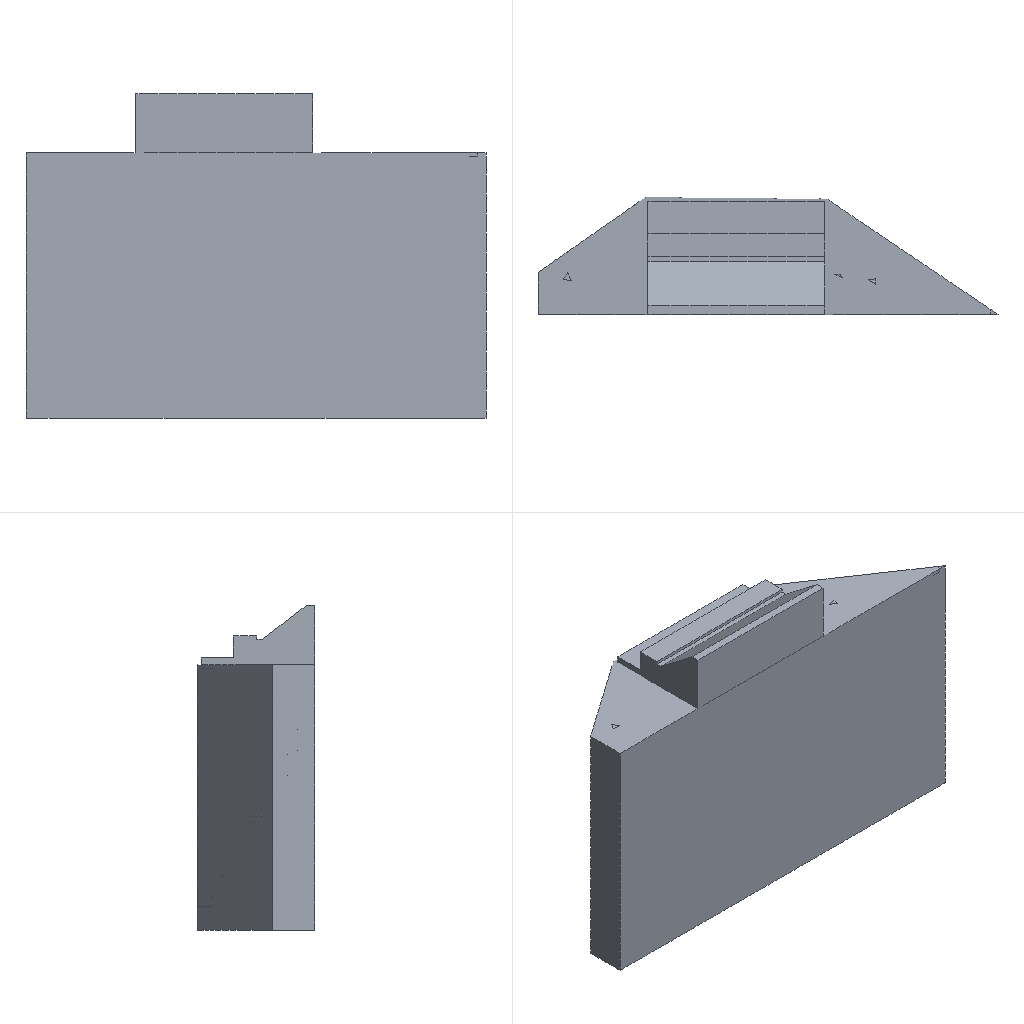Simulation study | ansys workbench
Set-up summary:
category,name,step,type,value,unit,region
solver,ansys_workbench
units,mm-N-s-tonne (MPa),,stated,"/units,MPA"
analysis,LS1,,static
load_step,LS1,LS1,static,nsubst=1; time=1
mesh,nodes,,,241341
mesh,elements,,,176783
element_type,SOLID187,,,141912
element_type,TARGE170,,,14127
element_type,CONTA174,,,14127
element_type,SOLID186,,,5881
element_type,SURF154,,,736
material,AC-16,,E,1300,tonne s^-2 mm^-1
material,AC-16,,nu,0.3
material,AC-16,,density,2.44e-09,tonne mm^-3
material,Water ?,,E,60,tonne s^-2 mm^-1
material,Water ?,,nu,0.3
material,Water ?,,density,1.9e-09,tonne mm^-3
material,C30,,E,30000,tonne s^-2 mm^-1
material,C30,,nu,0.2
material,C30,,density,2.6e-09,tonne mm^-3
material,SAM-13,,E,1800,tonne s^-2 mm^-1
material,SAM-13,,nu,0.33
material,SAM-13,,density,2.46e-09,tonne mm^-3
load,"Define Pressure Using Surface Effect Elements ""__""",LS1,pressure,0.5,,SURF154 #45
load,ACEL,LS1,gravity (ACEL; gravity acts opposite),"9806.65 [dir=(0, -1, 0)]",,all
bc,Fixed Supports,model,fixed,[dofs=ALL],,_FIXEDSU
contact,Contact Region,,bonded (always),element=CONTA174
contact,Contact Region 2,,bonded (always),element=CONTA174
contact,Contact Region 3,,bonded (always),element=CONTA174
contact,Contact Region 4,,bonded (always),element=CONTA174
contact,Contact Region 5,,bonded (always),element=CONTA174
contact,Contact Region 6,,bonded (always),element=CONTA174
contact,Contact Region 7,,bonded (always),element=CONTA174
contact,Contact Region 8,,bonded (always),element=CONTA174
contact,Contact Region 9,,bonded (always),element=CONTA174
contact,Contact Region 10,,bonded (always),element=CONTA174
contact,Contact Region 11,,bonded (always),element=CONTA174
contact,Contact Region 12,,bonded (always),element=CONTA174
contact,Contact Region 13,,bonded (always),element=CONTA174
contact,Contact Region 14,,bonded (always),element=CONTA174
contact,Contact Region 15,,bonded (always),element=CONTA174
contact,Contact Region 16,,bonded (always),element=CONTA174
contact,Contact Region 17,,bonded (always),element=CONTA174
named_set,_FIXEDSU,,node,7961
Ansys APDL input file, long lists of numbers shortened:
/batch
/config,noeldb,1     ! force off writing results to database
*get,_wallstrt,active,,time,wall
! ANSYS input file written by Workbench version 2024 R2
! File used for geometry attach:
/title,__--____ (A5)
! ****** Begin Custom Load Command Snippet ******
/COM, ACT Extensions:
/COM,     LSDYNA, 2024.2
/COM,/COM,     ANSYSMotion, 2024.2
/COM,
! ****** End   Custom Load Command Snippet ******
/com,--- Data in consistent NMM units. See Solving Units in the help system for more information.
/units,MPA
/nopr
/wb,file,start              !  signify a WB generated input file
/prep7
! Turn off shape checking because checks already performed inside WB mesher.
! See help system for more information.
SHPP,OFF,,NOWARN
/nolist
etcon,set             ! allow ANSYS to choose best KEYOP's for 180x elements, resets any applicable keyopt to MAPDL defaults
/com,*********** Nodes for the whole assembly ***********
nblock,3,,265475
(1i9,3e20.9e3)
   141650     3.031677267E+02     6.841687785E+02    -6.937544574E+02
! (241340 more lines like these left out)
-1
/wb,elem,start            !  set before creation of elements
/com,*********** Elements for Body 1 '62110001-FreeParts|__4[7]' ***********
et,1,186
keyo,1,2,1          ! set full integration on SOLID186
eblock,19,solid,,144
(19i9)
        1        1        1        1        0        0        0        0       20        0        1        1      194      199      201       92      195      200      224
! (287 more lines like these left out)
-1
/com,*********** Elements for Body 2 '62110001-FreeParts|__4[6]' ***********
et,2,186
keyo,2,2,1          ! set full integration on SOLID186
eblock,19,solid,,208
(19i9)
        2        2        2        2        0        0        0        0       20        0      145     1285     1317     1366     1392     1289     1316     1367     1393
! (415 more lines like these left out)
-1
/com,*********** Elements for Body 3 '62110001-FreeParts|__2' ***********
et,3,186
keyo,3,2,1          ! set full integration on SOLID186
eblock,19,solid,,1302
(19i9)
        3        3        3        3        0        0        0        0       20        0      353     3709     4247     4329     3762     3742     4307     4330     3763
! (2603 more lines like these left out)
-1
/com,*********** Elements for Body 4 '62110001-FreeParts|__4[2]' ***********
et,4,186
keyo,4,2,1          ! set full integration on SOLID186
eblock,19,solid,,1508
(19i9)
        4        4        4        4        0        0        0        0       20        0     1655     9285    11532    11587    11716     9986    11585    11586    11741
! (3015 more lines like these left out)
-1
/com,*********** Elements for Body 5 '62110001-FreeParts|__4[3]' ***********
et,5,186
keyo,5,2,1          ! set full integration on SOLID186
eblock,19,solid,,1392
(19i9)
        5        5        5        5        0        0        0        0       20        0     3163    18104    20284    20200    20142    19391    20307    20201    20170
! (2783 more lines like these left out)
-1
/com,*********** Elements for Body 6 '62110001-FreeParts|__3[6]' ***********
et,6,186
keyo,6,2,1          ! set full integration on SOLID186
eblock,19,solid,,591
(19i9)
        6        6        6        6        0        0        0        0       20        0     4555    26309    26310    26422    26421    27122    27121    27009    27010
! (1181 more lines like these left out)
-1
/com,*********** Elements for Body 7 '62110001-FreeParts|__4[5]' ***********
et,7,187
eblock,19,solid,,73405
(19i9)
        7        7        7        7        0        0        0        0       10        0     5146    37364    44991    40740    42244    97102   123084    97095    97098
! (146809 more lines like these left out)
-1
/com,*********** Elements for Body 8 '62110001-FreeParts|__4[4]' ***********
et,8,186
keyo,8,2,1          ! set full integration on SOLID186
eblock,19,solid,,667
(19i9)
        8        8        8        8        0        0        0        0       20        0    78551   137333   138129   138101   138099   137334   138005   138006   138007
! (1333 more lines like these left out)
-1
/com,*********** Elements for Body 9 '62110001-FreeParts|__4[8]' ***********
et,9,186
keyo,9,2,1          ! set full integration on SOLID186
eblock,19,solid,,69
(19i9)
        9        9        9        9        0        0        0        0       20        0    79218   141693   141815   141816   141817   141694   141764   141765   141740
! (137 more lines like these left out)
-1
/com,*********** Elements for Body 10 '62110001-FreeParts|__4[1]' ***********
et,10,187
eblock,19,solid,,68507
(19i9)
       10       10       10       10        0        0        0        0       10        0    79287   149696   150014   155698   150959   212844   215335   212849   212847
! (137013 more lines like these left out)
-1
/wb,elem,end               !  done creating elements
/com,*********** Send User Defined Coordinate System(s) ***********
csys,0
toffst,273.15,      ! Temperature offset from absolute zero
/com,*********** Set Reference Temperature ***********
tref,22.
/wb,mat,start              !  starting to send materials
/com,*********** Send Materials ***********
MP,DENS,1,2.44e-09,	! tonne mm^-3
MP,EX,1,1300,	! tonne s^-2 mm^-1
MP,NUXY,1,0.3,
! (36 more lines like these left out)
/wb,mat,end                !  done sending materials
!************************* Model Summary ********************
!62110001-FreeParts|åå²4[7],	AC-16,	matid,	1
!62110001-FreeParts|åå²4[6],	æ°´æ³¥å,	matid,	2
!62110001-FreeParts|ç»å2,	C30,	matid,	3
!62110001-FreeParts|åå²4[2],	æ°´æ³¥å,	matid,	4
!62110001-FreeParts|åå²4[3],	AC-16,	matid,	5
!62110001-FreeParts|åå²3[6],	C30,	matid,	6
!62110001-FreeParts|åå²4[5],	æ°´æ³¥å,	matid,	7
!62110001-FreeParts|åå²4[4],	SAM-13,	matid,	8
!62110001-FreeParts|åå²4[8],	SAM-13,	matid,	9
!62110001-FreeParts|åå²4[1],	æ°´æ³¥å,	matid,	10
!************************* End Model Summary ********************
! get the diagonal of the bounding box. Needed later for other things
*get,_xmin,node,,mnloc,x
*get,_ymin,node,,mnloc,y
*get,_zmin,node,,mnloc,z
*get,_xmax,node,,mxloc,x
*get,_ymax,node,,mxloc,y
*get,_zmax,node,,mxloc,z
_ASMDIAG=(_xmax-_xmin)*(_xmax-_xmin)+(_ymax-_ymin)*(_ymax-_ymin)+(_zmax-_zmin)*(_zmax-_zmin)
_ASMDIAG=SQRT(_ASMDIAG)
/wb,contact,start          !  starting to send contact
/com,*********** Create Contact "½Ó´¥ÇøÓò" ***********
/com,            Real Constant Set For Above Contact Is 12 & 11
*set,tid,12
*set,cid,11
r,tid
r,cid
et,tid,170
et,cid,174
eblock,10,,,72
(15i9)
   171066       12       12       12        0      191       93      188      192      630      629      843      849
! (71 more lines like these left out)
-1
eblock,10,,,72
(15i9)
   171138       11       11       11        0      191       93      188      192      630      629      843      849
! (71 more lines like these left out)
-1
eblock,10,,,78
(15i9)
   171210       11       12       11        0     1079     1082     1159     1078     1713     1719     1711     1710
! (77 more lines like these left out)
-1
eblock,10,,,78
(15i9)
   171288       12       11       12        0     1079     1082     1159     1078     1713     1719     1711     1710
! (77 more lines like these left out)
-1
keyo,cid,8,2               ! auto create asymmetric contact (from Program Controlled setting)
keyo,cid,10,0              ! adjust contact stiffness each NR iteration (from Program Controlled setting)
keyo,cid,12,5              ! bonded always
keyo,cid,18,1              ! small sliding turned on by application
keyo,cid,2,2               ! MPC for bonded contacts (from Program Controlled setting)
keyo,tid,5,0               ! Automatic constraint type detection
keyo,cid,4,2               ! on nodal point - normal to target surface (from Program Controlled setting)
keyo,cid,9,1               ! ignore initial gaps/penetration
keyo,cid,7,0               ! No Prediction
rmod,tid,3,10.      ! FKN
rmod,tid,5,0.       ! ICONT
rmod,tid,6,0.       ! PINB
rmod,tid,10,0.      ! CNOF
rmod,tid,12,0.      ! FKT
rmod,tid,36,269     ! WB DSID
rmod,cid,3,10.      ! FKN
rmod,cid,5,0.       ! ICONT
rmod,cid,6,0.       ! PINB
rmod,cid,10,0.      ! CNOF
rmod,cid,12,0.      ! FKT
rmod,cid,36,269     ! WB DSID
/com,*********** Create Contact "½Ó´¥ÇøÓò 2" ***********
/com,            Real Constant Set For Above Contact Is 14 & 13
*set,tid,14
*set,cid,13
r,tid
r,cid
et,tid,170
et,cid,174
eblock,10,,,48
(15i9)
   171366       14       14       14        0      142      249      295      141      752      940      750      749
! (47 more lines like these left out)
-1
eblock,10,,,48
(15i9)
   171414       13       13       13        0      142      249      295      141      752      940      750      749
! (47 more lines like these left out)
-1
eblock,10,,,48
(15i9)
   171462       13       14       13        0    20081    20262    20260    20111    25752    26053    25811    25751
! (47 more lines like these left out)
-1
eblock,10,,,48
(15i9)
   171510       14       13       14        0    20081    20262    20260    20111    25752    26053    25811    25751
! (47 more lines like these left out)
-1
keyo,cid,8,2               ! auto create asymmetric contact (from Program Controlled setting)
keyo,cid,10,0              ! adjust contact stiffness each NR iteration (from Program Controlled setting)
keyo,cid,12,5              ! bonded always
keyo,cid,18,1              ! small sliding turned on by application
keyo,cid,2,2               ! MPC for bonded contacts (from Program Controlled setting)
keyo,tid,5,0               ! Automatic constraint type detection
keyo,cid,4,2               ! on nodal point - normal to target surface (from Program Controlled setting)
keyo,cid,9,1               ! ignore initial gaps/penetration
keyo,cid,7,0               ! No Prediction
rmod,tid,3,10.      ! FKN
rmod,tid,5,0.       ! ICONT
rmod,tid,6,0.       ! PINB
rmod,tid,10,0.      ! CNOF
rmod,tid,12,0.      ! FKT
rmod,tid,36,272     ! WB DSID
rmod,cid,3,10.      ! FKN
rmod,cid,5,0.       ! ICONT
rmod,cid,6,0.       ! PINB
rmod,cid,10,0.      ! CNOF
rmod,cid,12,0.      ! FKT
rmod,cid,36,272     ! WB DSID
/com,*********** Create Contact "½Ó´¥ÇøÓò 3" ***********
/com,            Real Constant Set For Above Contact Is 16 & 15
*set,tid,16
*set,cid,15
r,tid
r,cid
et,tid,170
et,cid,174
eblock,10,,,72
(15i9)
   171558       16       16       16        0      224       92      195      200      626      625      858      865
! (71 more lines like these left out)
-1
eblock,10,,,72
(15i9)
   171630       15       15       15        0      224       92      195      200      626      625      858      865
! (71 more lines like these left out)
-1
eblock,10,,,69
(15i9)
   171702       15       16       15        0   141740   141694   141764   141765   142000   142001   142164   142116
! (68 more lines like these left out)
-1
eblock,10,,,69
(15i9)
   171771       16       15       16        0   141740   141694   141764   141765   142000   142001   142164   142116
! (68 more lines like these left out)
-1
keyo,cid,8,2               ! auto create asymmetric contact (from Program Controlled setting)
keyo,cid,10,0              ! adjust contact stiffness each NR iteration (from Program Controlled setting)
keyo,cid,12,5              ! bonded always
keyo,cid,18,1              ! small sliding turned on by application
keyo,cid,2,2               ! MPC for bonded contacts (from Program Controlled setting)
keyo,tid,5,0               ! Automatic constraint type detection
keyo,cid,4,2               ! on nodal point - normal to target surface (from Program Controlled setting)
keyo,cid,9,1               ! ignore initial gaps/penetration
keyo,cid,7,0               ! No Prediction
rmod,tid,3,10.      ! FKN
rmod,tid,5,0.       ! ICONT
rmod,tid,6,0.       ! PINB
rmod,tid,10,0.      ! CNOF
rmod,tid,12,0.      ! FKT
rmod,tid,36,275     ! WB DSID
rmod,cid,3,10.      ! FKN
rmod,cid,5,0.       ! ICONT
rmod,cid,6,0.       ! PINB
rmod,cid,10,0.      ! CNOF
rmod,cid,12,0.      ! FKT
rmod,cid,36,275     ! WB DSID
/com,*********** Create Contact "½Ó´¥ÇøÓò 4" ***********
/com,            Real Constant Set For Above Contact Is 18 & 17
*set,tid,18
*set,cid,17
r,tid
r,cid
et,tid,170
et,cid,174
eblock,10,,,104
(15i9)
   171840       18       18       18        0     1071     1342     1341     1072     1698     2330     1700     1697
! (103 more lines like these left out)
-1
eblock,10,,,104
(15i9)
   171944       17       17       17        0     1071     1342     1341     1072     1698     2330     1700     1697
! (103 more lines like these left out)
-1
eblock,10,,,104
(15i9)
   172048       17       18       17        0    11662    11613    11612    11663    17904    17901    17902    18000
! (103 more lines like these left out)
-1
eblock,10,,,104
(15i9)
   172152       18       17       18        0    11662    11613    11612    11663    17904    17901    17902    18000
! (103 more lines like these left out)
-1
keyo,cid,8,2               ! auto create asymmetric contact (from Program Controlled setting)
keyo,cid,10,0              ! adjust contact stiffness each NR iteration (from Program Controlled setting)
keyo,cid,12,5              ! bonded always
keyo,cid,18,1              ! small sliding turned on by application
keyo,cid,2,2               ! MPC for bonded contacts (from Program Controlled setting)
keyo,tid,5,0               ! Automatic constraint type detection
keyo,cid,4,2               ! on nodal point - normal to target surface (from Program Controlled setting)
keyo,cid,9,1               ! ignore initial gaps/penetration
keyo,cid,7,0               ! No Prediction
rmod,tid,3,10.      ! FKN
rmod,tid,5,0.       ! ICONT
rmod,tid,6,0.       ! PINB
rmod,tid,10,0.      ! CNOF
rmod,tid,12,0.      ! FKT
rmod,tid,36,278     ! WB DSID
rmod,cid,3,10.      ! FKN
rmod,cid,5,0.       ! ICONT
rmod,cid,6,0.       ! PINB
rmod,cid,10,0.      ! CNOF
rmod,cid,12,0.      ! FKT
rmod,cid,36,278     ! WB DSID
/com,*********** Create Contact "½Ó´¥ÇøÓò 5" ***********
/com,            Real Constant Set For Above Contact Is 20 & 19
*set,tid,20
*set,cid,19
r,tid
r,cid
et,tid,170
et,cid,174
eblock,10,,,130
(15i9)
   172256       20       20       20        0     1076     1186     1315     1077     1708     1949     1709     1707
! (129 more lines like these left out)
-1
eblock,10,,,130
(15i9)
   172386       19       19       19        0     1076     1186     1315     1077     1708     1949     1709     1707
! (129 more lines like these left out)
-1
eblock,10,,,220
(15i9)
   172516       19       20       19        0    34508    34518    34520    34520    73083    73157    34520    73085
! (219 more lines like these left out)
-1
eblock,10,,,220
(15i9)
   172736       20       19       20        0    34508    34518    34520    34520    73083    73157    34520    73085
! (219 more lines like these left out)
-1
keyo,cid,8,2               ! auto create asymmetric contact (from Program Controlled setting)
keyo,cid,10,0              ! adjust contact stiffness each NR iteration (from Program Controlled setting)
keyo,cid,12,5              ! bonded always
keyo,cid,18,1              ! small sliding turned on by application
keyo,cid,2,2               ! MPC for bonded contacts (from Program Controlled setting)
keyo,tid,5,0               ! Automatic constraint type detection
keyo,cid,4,2               ! on nodal point - normal to target surface (from Program Controlled setting)
keyo,cid,9,1               ! ignore initial gaps/penetration
keyo,cid,7,0               ! No Prediction
rmod,tid,3,10.      ! FKN
rmod,tid,5,0.       ! ICONT
rmod,tid,6,0.       ! PINB
rmod,tid,10,0.      ! CNOF
rmod,tid,12,0.      ! FKT
rmod,tid,36,281     ! WB DSID
rmod,cid,3,10.      ! FKN
rmod,cid,5,0.       ! ICONT
rmod,cid,6,0.       ! PINB
rmod,cid,10,0.      ! CNOF
rmod,cid,12,0.      ! FKT
rmod,cid,36,281     ! WB DSID
/com,*********** Create Contact "½Ó´¥ÇøÓò 6" ***********
/com,            Real Constant Set For Above Contact Is 22 & 21
*set,tid,22
*set,cid,21
r,tid
r,cid
et,tid,170
et,cid,174
eblock,10,,,315
(15i9)
   172956       22       22       22        0     3729     3449     3765     3764     7481     7482     8199     8140
! (314 more lines like these left out)
-1
eblock,10,,,315
(15i9)
   173271       21       21       21        0     3729     3449     3765     3764     7481     7482     8199     8140
! (314 more lines like these left out)
-1
eblock,10,,,329
(15i9)
   173586       21       22       21        0    26709    26657    26710    26710    29003    29004    26710    29122
! (328 more lines like these left out)
-1
eblock,10,,,329
(15i9)
   173915       22       21       22        0    26709    26657    26710    26710    29003    29004    26710    29122
! (328 more lines like these left out)
-1
keyo,cid,8,2               ! auto create asymmetric contact (from Program Controlled setting)
keyo,cid,10,0              ! adjust contact stiffness each NR iteration (from Program Controlled setting)
keyo,cid,12,5              ! bonded always
keyo,cid,18,1              ! small sliding turned on by application
keyo,cid,2,0               ! augmented Lagrange (from Program Controlled setting)
keyo,cid,4,0               ! on Gauss point (from Program Controlled setting)
keyo,cid,9,1               ! ignore initial gaps/penetration
keyo,cid,7,0               ! No Prediction
rmod,tid,3,10.      ! FKN
rmod,tid,5,0.       ! ICONT
rmod,tid,6,0.       ! PINB
rmod,tid,10,0.      ! CNOF
rmod,tid,12,0.      ! FKT
rmod,tid,36,284     ! WB DSID
rmod,cid,3,10.      ! FKN
rmod,cid,5,0.       ! ICONT
rmod,cid,6,0.       ! PINB
rmod,cid,10,0.      ! CNOF
rmod,cid,12,0.      ! FKT
rmod,cid,36,284     ! WB DSID
/com,*********** Create Contact "½Ó´¥ÇøÓò 7" ***********
/com,            Real Constant Set For Above Contact Is 24 & 23
*set,tid,24
*set,cid,23
r,tid
r,cid
et,tid,170
et,cid,174
eblock,10,,,780
(15i9)
   174244       24       24       24        0    10048    10078    10857    10047    14730    14790    14728    14727
! (779 more lines like these left out)
-1
eblock,10,,,780
(15i9)
   175024       23       23       23        0    10048    10078    10857    10047    14730    14790    14728    14727
! (779 more lines like these left out)
-1
eblock,10,,,696
(15i9)
   175804       23       24       23        0    20059    19392    20140    20141    24322    24323    25868    25707
! (695 more lines like these left out)
-1
eblock,10,,,696
(15i9)
   176500       24       23       24        0    20059    19392    20140    20141    24322    24323    25868    25707
! (695 more lines like these left out)
-1
keyo,cid,8,2               ! auto create asymmetric contact (from Program Controlled setting)
keyo,cid,10,0              ! adjust contact stiffness each NR iteration (from Program Controlled setting)
keyo,cid,12,5              ! bonded always
keyo,cid,18,1              ! small sliding turned on by application
keyo,cid,2,2               ! MPC for bonded contacts (from Program Controlled setting)
keyo,tid,5,0               ! Automatic constraint type detection
keyo,cid,4,2               ! on nodal point - normal to target surface (from Program Controlled setting)
keyo,cid,9,1               ! ignore initial gaps/penetration
keyo,cid,7,0               ! No Prediction
rmod,tid,3,10.      ! FKN
rmod,tid,5,0.       ! ICONT
rmod,tid,6,0.       ! PINB
rmod,tid,10,0.      ! CNOF
rmod,tid,12,0.      ! FKT
rmod,tid,36,287     ! WB DSID
rmod,cid,3,10.      ! FKN
rmod,cid,5,0.       ! ICONT
rmod,cid,6,0.       ! PINB
rmod,cid,10,0.      ! CNOF
rmod,cid,12,0.      ! FKT
rmod,cid,36,287     ! WB DSID
/com,*********** Create Contact "½Ó´¥ÇøÓò 8" ***********
/com,            Real Constant Set For Above Contact Is 26 & 25
*set,tid,26
*set,cid,25
r,tid
r,cid
et,tid,170
et,cid,174
eblock,10,,,52
(15i9)
   177196       26       26       26        0    11587    11716    11741    11586    17853    18080    17851    17850
! (51 more lines like these left out)
-1
eblock,10,,,52
(15i9)
   177248       25       25       25        0    11587    11716    11741    11586    17853    18080    17851    17850
! (51 more lines like these left out)
-1
eblock,10,,,76
(15i9)
   177300       25       26       25        0    26927    27028    27027    26963    29676    29878    29749    29675
! (75 more lines like these left out)
-1
eblock,10,,,76
(15i9)
   177376       26       25       26        0    26927    27028    27027    26963    29676    29878    29749    29675
! (75 more lines like these left out)
-1
keyo,cid,8,2               ! auto create asymmetric contact (from Program Controlled setting)
keyo,cid,10,0              ! adjust contact stiffness each NR iteration (from Program Controlled setting)
keyo,cid,12,5              ! bonded always
keyo,cid,18,1              ! small sliding turned on by application
keyo,cid,2,0               ! augmented Lagrange (from Program Controlled setting)
keyo,cid,4,0               ! on Gauss point (from Program Controlled setting)
keyo,cid,9,1               ! ignore initial gaps/penetration
keyo,cid,7,0               ! No Prediction
rmod,tid,3,10.      ! FKN
rmod,tid,5,0.       ! ICONT
rmod,tid,6,0.       ! PINB
rmod,tid,10,0.      ! CNOF
rmod,tid,12,0.      ! FKT
rmod,tid,36,290     ! WB DSID
rmod,cid,3,10.      ! FKN
rmod,cid,5,0.       ! ICONT
rmod,cid,6,0.       ! PINB
rmod,cid,10,0.      ! CNOF
rmod,cid,12,0.      ! FKT
rmod,cid,36,290     ! WB DSID
/com,*********** Create Contact "½Ó´¥ÇøÓò 9" ***********
/com,            Real Constant Set For Above Contact Is 28 & 27
*set,tid,28
*set,cid,27
r,tid
r,cid
et,tid,170
et,cid,174
eblock,10,,,52
(15i9)
   177452       28       28       28        0    11714    11664    11689    11715    18005    18004    18053    18078
! (51 more lines like these left out)
-1
eblock,10,,,52
(15i9)
   177504       27       27       27        0    11714    11664    11689    11715    18005    18004    18053    18078
! (51 more lines like these left out)
-1
eblock,10,,,111
(15i9)
   177556       27       28       27        0    34507    34569    34523    34523    73077    73189    34523    73074
! (110 more lines like these left out)
-1
eblock,10,,,111
(15i9)
   177667       28       27       28        0    34507    34569    34523    34523    73077    73189    34523    73074
! (110 more lines like these left out)
-1
keyo,cid,8,2               ! auto create asymmetric contact (from Program Controlled setting)
keyo,cid,10,0              ! adjust contact stiffness each NR iteration (from Program Controlled setting)
keyo,cid,12,5              ! bonded always
keyo,cid,18,1              ! small sliding turned on by application
keyo,cid,2,2               ! MPC for bonded contacts (from Program Controlled setting)
keyo,tid,5,0               ! Automatic constraint type detection
keyo,cid,4,2               ! on nodal point - normal to target surface (from Program Controlled setting)
keyo,cid,9,1               ! ignore initial gaps/penetration
keyo,cid,7,0               ! No Prediction
rmod,tid,3,10.      ! FKN
rmod,tid,5,0.       ! ICONT
rmod,tid,6,0.       ! PINB
rmod,tid,10,0.      ! CNOF
rmod,tid,12,0.      ! FKT
rmod,tid,36,293     ! WB DSID
rmod,cid,3,10.      ! FKN
rmod,cid,5,0.       ! ICONT
rmod,cid,6,0.       ! PINB
rmod,cid,10,0.      ! CNOF
rmod,cid,12,0.      ! FKT
rmod,cid,36,293     ! WB DSID
/com,*********** Create Contact "½Ó´¥ÇøÓò 10" ***********
/com,            Real Constant Set For Above Contact Is 30 & 29
*set,tid,30
*set,cid,29
r,tid
r,cid
et,tid,170
et,cid,174
eblock,10,,,728
(15i9)
   177778       30       30       30        0    11611    10884    10019    10018    16449    14673    14670    14671
! (727 more lines like these left out)
-1
eblock,10,,,728
(15i9)
   178506       29       29       29        0    11611    10884    10019    10018    16449    14673    14670    14671
! (727 more lines like these left out)
-1
eblock,10,,,1574
(15i9)
   179234       29       30       29        0   145335   145445   145448   145448   178055   179093   145448   178056
! (1573 more lines like these left out)
-1
eblock,10,,,1574
(15i9)
   180808       30       29       30        0   145335   145445   145448   145448   178055   179093   145448   178056
! (1573 more lines like these left out)
-1
keyo,cid,8,2               ! auto create asymmetric contact (from Program Controlled setting)
keyo,cid,10,0              ! adjust contact stiffness each NR iteration (from Program Controlled setting)
keyo,cid,12,5              ! bonded always
keyo,cid,18,1              ! small sliding turned on by application
keyo,cid,2,2               ! MPC for bonded contacts (from Program Controlled setting)
keyo,tid,5,0               ! Automatic constraint type detection
keyo,cid,4,2               ! on nodal point - normal to target surface (from Program Controlled setting)
keyo,cid,9,1               ! ignore initial gaps/penetration
keyo,cid,7,0               ! No Prediction
rmod,tid,3,10.      ! FKN
rmod,tid,5,0.       ! ICONT
rmod,tid,6,0.       ! PINB
rmod,tid,10,0.      ! CNOF
rmod,tid,12,0.      ! FKT
rmod,tid,36,296     ! WB DSID
rmod,cid,3,10.      ! FKN
rmod,cid,5,0.       ! ICONT
rmod,cid,6,0.       ! PINB
rmod,cid,10,0.      ! CNOF
rmod,cid,12,0.      ! FKT
rmod,cid,36,296     ! WB DSID
/com,*********** Create Contact "½Ó´¥ÇøÓò 11" ***********
/com,            Real Constant Set For Above Contact Is 32 & 31
*set,tid,32
*set,cid,31
r,tid
r,cid
et,tid,170
et,cid,174
eblock,10,,,48
(15i9)
   182382       32       32       32        0    20036    20308    20198    20112    25661    25958    25813    25660
! (47 more lines like these left out)
-1
eblock,10,,,48
(15i9)
   182430       31       31       31        0    20036    20308    20198    20112    25661    25958    25813    25660
! (47 more lines like these left out)
-1
eblock,10,,,53
(15i9)
   182478       31       32       31        0    27027    27139    27241    27026    29879    30113    29877    29875
! (52 more lines like these left out)
-1
eblock,10,,,53
(15i9)
   182531       32       31       32        0    27027    27139    27241    27026    29879    30113    29877    29875
! (52 more lines like these left out)
-1
keyo,cid,8,2               ! auto create asymmetric contact (from Program Controlled setting)
keyo,cid,10,0              ! adjust contact stiffness each NR iteration (from Program Controlled setting)
keyo,cid,12,5              ! bonded always
keyo,cid,18,1              ! small sliding turned on by application
keyo,cid,2,0               ! augmented Lagrange (from Program Controlled setting)
keyo,cid,4,0               ! on Gauss point (from Program Controlled setting)
keyo,cid,9,1               ! ignore initial gaps/penetration
keyo,cid,7,0               ! No Prediction
rmod,tid,3,10.      ! FKN
rmod,tid,5,0.       ! ICONT
rmod,tid,6,0.       ! PINB
rmod,tid,10,0.      ! CNOF
rmod,tid,12,0.      ! FKT
rmod,tid,36,299     ! WB DSID
rmod,cid,3,10.      ! FKN
rmod,cid,5,0.       ! ICONT
rmod,cid,6,0.       ! PINB
rmod,cid,10,0.      ! CNOF
rmod,cid,12,0.      ! FKT
rmod,cid,36,299     ! WB DSID
/com,*********** Create Contact "½Ó´¥ÇøÓò 12" ***********
/com,            Real Constant Set For Above Contact Is 34 & 33
*set,tid,34
*set,cid,33
r,tid
r,cid
et,tid,170
et,cid,174
eblock,10,,,696
(15i9)
   182584       34       34       34        0    20170    19391    20307    20201    24318    24319    25962    25929
! (695 more lines like these left out)
-1
eblock,10,,,696
(15i9)
   183280       33       33       33        0    20170    19391    20307    20201    24318    24319    25962    25929
! (695 more lines like these left out)
-1
eblock,10,,,667
(15i9)
   183976       33       34       33        0   138007   137334   138005   138006   140059   140058   141450   141452
! (666 more lines like these left out)
-1
eblock,10,,,667
(15i9)
   184643       34       33       34        0   138007   137334   138005   138006   140059   140058   141450   141452
! (666 more lines like these left out)
-1
keyo,cid,8,2               ! auto create asymmetric contact (from Program Controlled setting)
keyo,cid,10,0              ! adjust contact stiffness each NR iteration (from Program Controlled setting)
keyo,cid,12,5              ! bonded always
keyo,cid,18,1              ! small sliding turned on by application
keyo,cid,2,2               ! MPC for bonded contacts (from Program Controlled setting)
keyo,tid,5,0               ! Automatic constraint type detection
keyo,cid,4,2               ! on nodal point - normal to target surface (from Program Controlled setting)
keyo,cid,9,1               ! ignore initial gaps/penetration
keyo,cid,7,0               ! No Prediction
rmod,tid,3,10.      ! FKN
rmod,tid,5,0.       ! ICONT
rmod,tid,6,0.       ! PINB
rmod,tid,10,0.      ! CNOF
rmod,tid,12,0.      ! FKT
rmod,tid,36,302     ! WB DSID
rmod,cid,3,10.      ! FKN
rmod,cid,5,0.       ! ICONT
rmod,cid,6,0.       ! PINB
rmod,cid,10,0.      ! CNOF
rmod,cid,12,0.      ! FKT
rmod,cid,36,302     ! WB DSID
/com,*********** Create Contact "½Ó´¥ÇøÓò 13" ***********
/com,            Real Constant Set For Above Contact Is 36 & 35
*set,tid,36
*set,cid,35
r,tid
r,cid
et,tid,170
et,cid,174
eblock,10,,,48
(15i9)
   185310       36       36       36        0    20081    20262    20260    20111    25752    26053    25811    25751
! (47 more lines like these left out)
-1
eblock,10,,,48
(15i9)
   185358       35       35       35        0    20081    20262    20260    20111    25752    26053    25811    25751
! (47 more lines like these left out)
-1
eblock,10,,,23
(15i9)
   185406       35       36       35        0   141790   141788   141789   141812   142212   142211   142213   142215
! (22 more lines like these left out)
-1
eblock,10,,,23
(15i9)
   185429       36       35       36        0   141790   141788   141789   141812   142212   142211   142213   142215
! (22 more lines like these left out)
-1
keyo,cid,8,2               ! auto create asymmetric contact (from Program Controlled setting)
keyo,cid,10,0              ! adjust contact stiffness each NR iteration (from Program Controlled setting)
keyo,cid,12,5              ! bonded always
keyo,cid,18,1              ! small sliding turned on by application
keyo,cid,2,2               ! MPC for bonded contacts (from Program Controlled setting)
keyo,tid,5,0               ! Automatic constraint type detection
keyo,cid,4,2               ! on nodal point - normal to target surface (from Program Controlled setting)
keyo,cid,9,1               ! ignore initial gaps/penetration
keyo,cid,7,0               ! No Prediction
rmod,tid,3,10.      ! FKN
rmod,tid,5,0.       ! ICONT
rmod,tid,6,0.       ! PINB
rmod,tid,10,0.      ! CNOF
rmod,tid,12,0.      ! FKT
rmod,tid,36,305     ! WB DSID
rmod,cid,3,10.      ! FKN
rmod,cid,5,0.       ! ICONT
rmod,cid,6,0.       ! PINB
rmod,cid,10,0.      ! CNOF
rmod,cid,12,0.      ! FKT
rmod,cid,36,305     ! WB DSID
/com,*********** Create Contact "½Ó´¥ÇøÓò 14" ***********
/com,            Real Constant Set For Above Contact Is 38 & 37
*set,tid,38
*set,cid,37
r,tid
r,cid
et,tid,170
et,cid,174
eblock,10,,,29
(15i9)
   185452       38       38       38        0    27047    27159    27158    27046    29919    30151    29917    29916
! (28 more lines like these left out)
-1
eblock,10,,,29
(15i9)
   185481       37       37       37        0    27047    27159    27158    27046    29919    30151    29917    29916
! (28 more lines like these left out)
-1
eblock,10,,,23
(15i9)
   185510       37       38       37        0   138054   138052   138053   138076   141544   141543   141545   141547
! (22 more lines like these left out)
-1
eblock,10,,,23
(15i9)
   185533       38       37       38        0   138054   138052   138053   138076   141544   141543   141545   141547
! (22 more lines like these left out)
-1
keyo,cid,8,2               ! auto create asymmetric contact (from Program Controlled setting)
keyo,cid,10,0              ! adjust contact stiffness each NR iteration (from Program Controlled setting)
keyo,cid,12,5              ! bonded always
keyo,cid,18,1              ! small sliding turned on by application
keyo,cid,2,0               ! augmented Lagrange (from Program Controlled setting)
keyo,cid,4,0               ! on Gauss point (from Program Controlled setting)
keyo,cid,9,1               ! ignore initial gaps/penetration
keyo,cid,7,0               ! No Prediction
rmod,tid,3,10.      ! FKN
rmod,tid,5,0.       ! ICONT
rmod,tid,6,0.       ! PINB
rmod,tid,10,0.      ! CNOF
rmod,tid,12,0.      ! FKT
rmod,tid,36,308     ! WB DSID
rmod,cid,3,10.      ! FKN
rmod,cid,5,0.       ! ICONT
rmod,cid,6,0.       ! PINB
rmod,cid,10,0.      ! CNOF
rmod,cid,12,0.      ! FKT
rmod,cid,36,308     ! WB DSID
/com,*********** Create Contact "½Ó´¥ÇøÓò 15" ***********
/com,            Real Constant Set For Above Contact Is 40 & 39
*set,tid,40
*set,cid,39
r,tid
r,cid
et,tid,170
et,cid,174
eblock,10,,,568
(15i9)
   185556       40       40       40        0    26722    26721    26774    26774    29148    29151    26774    29154
! (567 more lines like these left out)
-1
eblock,10,,,568
(15i9)
   186124       39       39       39        0    26722    26721    26774    26774    29148    29151    26774    29154
! (567 more lines like these left out)
-1
eblock,10,,,1078
(15i9)
   186692       39       40       39        0   144057   144242   144139   144139   169853   170561   144139   169851
! (1077 more lines like these left out)
-1
eblock,10,,,1078
(15i9)
   187770       40       39       40        0   144057   144242   144139   144139   169853   170561   144139   169851
! (1077 more lines like these left out)
-1
keyo,cid,8,2               ! auto create asymmetric contact (from Program Controlled setting)
keyo,cid,10,0              ! adjust contact stiffness each NR iteration (from Program Controlled setting)
keyo,cid,12,5              ! bonded always
keyo,cid,18,1              ! small sliding turned on by application
keyo,cid,2,0               ! augmented Lagrange (from Program Controlled setting)
keyo,cid,4,0               ! on Gauss point (from Program Controlled setting)
keyo,cid,9,1               ! ignore initial gaps/penetration
keyo,cid,7,0               ! No Prediction
rmod,tid,3,10.      ! FKN
rmod,tid,5,0.       ! ICONT
rmod,tid,6,0.       ! PINB
rmod,tid,10,0.      ! CNOF
rmod,tid,12,0.      ! FKT
rmod,tid,36,311     ! WB DSID
rmod,cid,3,10.      ! FKN
rmod,cid,5,0.       ! ICONT
rmod,cid,6,0.       ! PINB
rmod,cid,10,0.      ! CNOF
rmod,cid,12,0.      ! FKT
rmod,cid,36,311     ! WB DSID
/com,*********** Create Contact "½Ó´¥ÇøÓò 16" ***********
/com,            Real Constant Set For Above Contact Is 42 & 41
*set,tid,42
*set,cid,41
r,tid
r,cid
et,tid,170
et,cid,174
eblock,10,,,2595
(15i9)
   188848       42       42       42        0    30686    30718    30742    30742    45416    45741    30742    45417
! (2594 more lines like these left out)
-1
eblock,10,,,2595
(15i9)
   191443       41       41       41        0    30686    30718    30742    30742    45416    45741    30742    45417
! (2594 more lines like these left out)
-1
eblock,10,,,2595
(15i9)
   194038       41       42       41        0   142320   142381   142321   142321   156095   156101   142321   156094
! (2594 more lines like these left out)
-1
eblock,10,,,2595
(15i9)
   196633       42       41       42        0   142320   142381   142321   142321   156095   156101   142321   156094
! (2594 more lines like these left out)
-1
keyo,cid,8,2               ! auto create asymmetric contact (from Program Controlled setting)
keyo,cid,10,0              ! adjust contact stiffness each NR iteration (from Program Controlled setting)
keyo,cid,12,5              ! bonded always
keyo,cid,18,1              ! small sliding turned on by application
keyo,cid,2,0               ! augmented Lagrange (from Program Controlled setting)
keyo,cid,4,0               ! on Gauss point (from Program Controlled setting)
keyo,cid,9,1               ! ignore initial gaps/penetration
keyo,cid,7,0               ! No Prediction
rmod,tid,3,10.      ! FKN
rmod,tid,5,0.       ! ICONT
rmod,tid,6,0.       ! PINB
rmod,tid,10,0.      ! CNOF
rmod,tid,12,0.      ! FKT
rmod,tid,36,314     ! WB DSID
rmod,cid,3,10.      ! FKN
rmod,cid,5,0.       ! ICONT
rmod,cid,6,0.       ! PINB
rmod,cid,10,0.      ! CNOF
rmod,cid,12,0.      ! FKT
rmod,cid,36,314     ! WB DSID
/com,*********** Create Contact "½Ó´¥ÇøÓò 17" ***********
/com,            Real Constant Set For Above Contact Is 44 & 43
*set,tid,44
*set,cid,43
r,tid
r,cid
et,tid,170
et,cid,174
eblock,10,,,23
(15i9)
   199228       44       44       44        0   138101   138099   138007   138006   141593   141455   141452   141453
! (22 more lines like these left out)
-1
eblock,10,,,23
(15i9)
   199251       43       43       43        0   138101   138099   138007   138006   141593   141455   141452   141453
! (22 more lines like these left out)
-1
eblock,10,,,23
(15i9)
   199274       43       44       43        0   141790   141788   141789   141812   142212   142211   142213   142215
! (22 more lines like these left out)
-1
eblock,10,,,23
(15i9)
   199297       44       43       44        0   141790   141788   141789   141812   142212   142211   142213   142215
! (22 more lines like these left out)
-1
keyo,cid,8,2               ! auto create asymmetric contact (from Program Controlled setting)
keyo,cid,10,0              ! adjust contact stiffness each NR iteration (from Program Controlled setting)
keyo,cid,12,5              ! bonded always
keyo,cid,18,1              ! small sliding turned on by application
keyo,cid,2,2               ! MPC for bonded contacts (from Program Controlled setting)
keyo,tid,5,0               ! Automatic constraint type detection
keyo,cid,4,2               ! on nodal point - normal to target surface (from Program Controlled setting)
keyo,cid,9,1               ! ignore initial gaps/penetration
keyo,cid,7,0               ! No Prediction
rmod,tid,3,10.      ! FKN
rmod,tid,5,0.       ! ICONT
rmod,tid,6,0.       ! PINB
rmod,tid,10,0.      ! CNOF
rmod,tid,12,0.      ! FKT
rmod,tid,36,317     ! WB DSID
rmod,cid,3,10.      ! FKN
rmod,cid,5,0.       ! ICONT
rmod,cid,6,0.       ! PINB
rmod,cid,10,0.      ! CNOF
rmod,cid,12,0.      ! FKT
rmod,cid,36,317     ! WB DSID
nsel,all
esel,all
/wb,contact,end            !  done creating contacts
/golist
/wb,load,start             !  starting to send loads
/com,*********** Fixed Supports ***********
CMBLOCK,_FIXEDSU,NODE,     7961
(8i10)
      3428      3429      3430      3431      3432      3448      3764      3765
! (995 more lines like these left out)
cmsel,s,_FIXEDSU
d,all,all
nsel,all
/com,*********** Define Pressure Using Surface Effect Elements "__" ***********
et,45,154
mat,45
eblock,10,,,736
(15i9)
   199320       45       45       45        0   138129   137333   138099   138101   140055   140054   141593   141595
! (735 more lines like these left out)
-1
esel,s,type,,45
keyop,45,7,0        ! Use deformed area for application of load
esel,all
esel,all
/gst,on,on
fini
*get,_numnode,node,0,count
*get,_numelem,elem,0,count
*get, _MAXELEMNUM, elem, 0, NUM, MAX
*get, _MAXNODENUM, node, 0, NUM, MAX
*get, _MAXELEMTYPE, etyp, 0, NUM, MAX
*get, _MAXREALCONST, rcon, 0, NUM, MAX
/go
/wb,load,end               !  done creating loads
/com,--- Number of total nodes = %_numnode%
/com,--- Number of contact elements = 28990
/com,--- Number of spring elements = 0
/com,--- Number of bearing elements = 0
/com,--- Number of solid elements = 147793
/com,--- Number of condensed parts = 0
/com,--- Number of total elements = %_numelem%
*get,_wallbsol,active,,time,wall
/com,****************************************************************************
/com,*************************    SOLUTION       ********************************
/com,****************************************************************************
/solu
antype,0                   ! static analysis
_thickRatio=0.3     ! Ratio of thick parts in the model
eqsl,sparse,,,,,1
cntr,print,1               ! print out contact info and also make no initial contact an error
dmpoption,emat,no             ! Don't combine emat file for DANSYS
dmpoption,esav,no             ! Don't combine esav file for DANSYS
nldiag,cont,iter           ! print out contact info each equilibrium iteration
rescontrol,,none                 ! Do not keep any restart files
/com,****************************************************
/com,******************* SOLVE FOR LS 1 OF 1 ****************
esel,s,type,,45
nsle
sf,all,pres,0.5
nsel,all
esel,all
acel,0.,9806.65,0.
esel,all
/nopr
/gopr
nsub,1,1,1
time,1.
outres,erase
outres,all,none
outres,nsol,all,
outres,rsol,all
outres,eangl,all
outres,etmp,all
outres,veng,all
outres,strs,all,
outres,epel,all,
outres,eppl,all,
outres,cont,all,
! *********** WB SOLVE COMMAND ***********
! check interactive state
*get,ANSINTER_,active,,int
*if,ANSINTER_,ne,0,then
/eof
*endif
solve
/com *************** Write FE CONNECTORS *********
CEWRITE,file,ce,,INTE
/com,****************************************************
/com,*************** FINISHED SOLVE FOR LS 1 *************
*get,_wallasol,active,,time,wall
/nopr
*get,_numnode,node,0,count
*get,_numelem,elem,0,count
*get, _MAXELEMNUM, elem, 0, NUM, MAX
*get, _MAXNODENUM, node, 0, NUM, MAX,,,INTERNAL
*get, _MAXELEMTYPE, etyp, 0, NUM, MAX
*get, _MAXREALCONST, rcon, 0, NUM, MAX
*get,_NSOLTHREADS,active,0,ntfs
*get,_NSOLPROCESSES,active,0,npfs
/gopr
/post1
xmlo,ENCODING,ISO-8859-1
xmlo,parm
/xml,parm,xml
fini
/gopr
*get,_walldone,active,,time,wall
_preptime=(_wallbsol-_wallstrt)*3600
_solvtime=(_wallasol-_wallbsol)*3600
_posttime=(_walldone-_wallasol)*3600
_totaltim=(_walldone-_wallstrt)*3600
*get,_dlbratio,active,0,solu,dlbr
*get,_combtime,active,0,solu,comb
*get,_ssmode,active,0,solu,ssmm
*get,_ndofs,active,0,solu,ndof
*get,_sol_end_time,active,0,set,time
*if,_sol_end_time,eq,1.,then
/fclean				!clean distributed files
*endif
/com,--- Total number of nodes = %_numnode%
/com,--- Total number of elements = %_numelem%
/com,--- Element load balance ratio = %_dlbratio%
/com,--- Time to combine distributed files = %_combtime%
/com,--- Sparse memory mode = %_ssmode%
/com,--- Number of DOF = %_ndofs%
/wb,file,end               ! done with WB generated input
Results summary:
result,analyses[0].index,,,1
result,analyses[0].system,,,SYS
result,analyses[0].deck,,,deck.dat
result,analyses[0].solve_status,,,completed
result,analyses[0].analysis_type,,,static
result,analyses[0].physics,,,mechanical
result,analyses[0].unit_system,,,"NMM: mm, ton, N, s, mV, mA, degC"
result,analyses[0].n_sets,,,1
result,analyses[0].load_steps[0].set,set=1,,1
result,analyses[0].load_steps[0].time_or_freq,set=1,,1
result,analyses[0].load_steps[0].max_displacement_magnitude,set=1,,4.92
result,analyses[0].load_steps[0].max_von_mises_nodal,set=1,,22.613
result,analyses[0].load_steps[0].reaction_force_sum_xyz[1],set=1,,8806.18
result,analyses[0].load_steps[0].reaction_force_sum_xyz[2],set=1,,880697
result,analyses[0].load_steps[0].reaction_force_sum_xyz[3],set=1,,-2.56161e-06